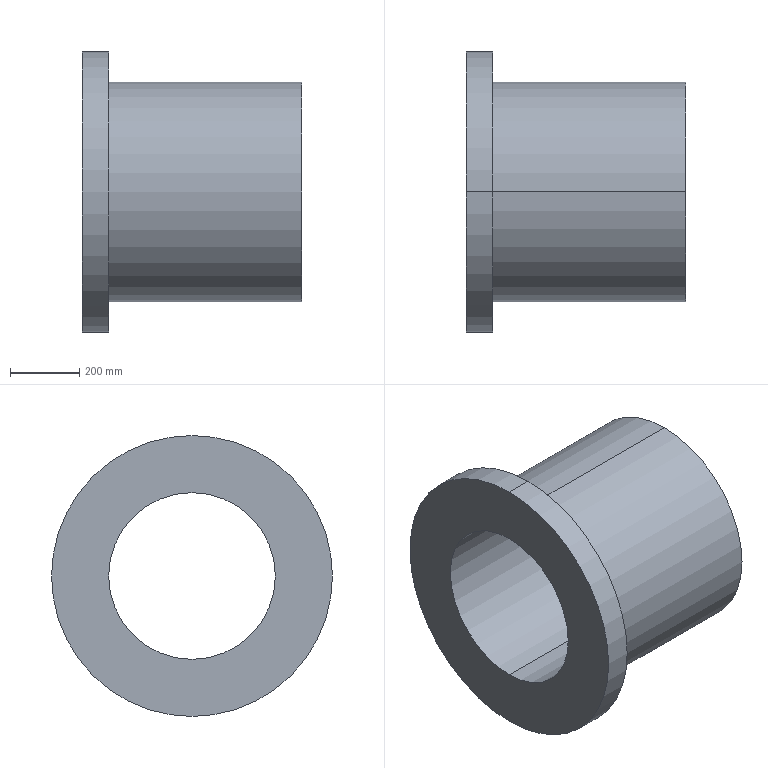Part | SolidWorks | features Revolution 1 | 1 solid | 9 faces | box 635 x 812.8 x 812.8 mm | volume 100350275 mm3 | cylinder 6 | plane 3 | commonest cylinder face diameters 482.6 x2 635 x2 812.8 x2
STEP:
#1=CARTESIAN_POINT('',(3.,0.,16.));
#2=VERTEX_POINT('',#1);
#3=CARTESIAN_POINT('',(3.,0.,-16.));
#4=VERTEX_POINT('',#3);
#5=CARTESIAN_POINT('',(3.,0.,0.));
#6=DIRECTION('',(-1.,0.,0.));
#7=DIRECTION('',(0.,0.,1.));
#8=AXIS2_PLACEMENT_3D('',#5,#6,#7);
#9=CIRCLE('',#8,16.);
#10=EDGE_CURVE('',#2,#4,#9,.T.);
#11=ORIENTED_EDGE('',*,*,#10,.T.);
#12=CARTESIAN_POINT('',(0.,0.,-16.));
#13=VERTEX_POINT('',#12);
#14=CARTESIAN_POINT('',(0.,0.,-16.));
#15=DIRECTION('',(-1.,0.,0.));
#16=VECTOR('',#15,39.37);
#17=LINE('',#14,#16);
#18=EDGE_CURVE('',#4,#13,#17,.T.);
#19=ORIENTED_EDGE('',*,*,#18,.T.);
#20=CARTESIAN_POINT('',(0.,0.,16.));
#21=VERTEX_POINT('',#20);
#22=CARTESIAN_POINT('',(0.,0.,0.));
#23=DIRECTION('',(-1.,0.,0.));
#24=DIRECTION('',(0.,0.,1.));
#25=AXIS2_PLACEMENT_3D('',#22,#23,#24);
#26=CIRCLE('',#25,16.);
#27=EDGE_CURVE('',#21,#13,#26,.T.);
#28=ORIENTED_EDGE('',*,*,#27,.F.);
#29=CARTESIAN_POINT('',(0.,0.,16.));
#30=DIRECTION('',(-1.,0.,0.));
#31=VECTOR('',#30,39.37);
#32=LINE('',#29,#31);
#33=EDGE_CURVE('',#2,#21,#32,.T.);
#34=ORIENTED_EDGE('',*,*,#33,.F.);
#35=EDGE_LOOP('',(#11,#19,#28,#34));
#36=FACE_OUTER_BOUND('',#35,.T.);
#37=CARTESIAN_POINT('',(0.,0.,0.));
#38=DIRECTION('',(-1.,0.,0.));
#39=DIRECTION('',(0.,0.,1.));
#40=AXIS2_PLACEMENT_3D('',#37,#38,#39);
#41=CYLINDRICAL_SURFACE('',#40,16.);
#42=ADVANCED_FACE('',(#36),#41,.T.);
#43=CARTESIAN_POINT('',(25.,0.,12.5));
#44=VERTEX_POINT('',#43);
#45=CARTESIAN_POINT('',(25.,0.,-12.5));
#46=VERTEX_POINT('',#45);
#47=CARTESIAN_POINT('',(25.,0.,0.));
#48=DIRECTION('',(-1.,0.,0.));
#49=DIRECTION('',(0.,0.,1.));
#50=AXIS2_PLACEMENT_3D('',#47,#48,#49);
#51=CIRCLE('',#50,12.5);
#52=EDGE_CURVE('',#44,#46,#51,.T.);
#53=ORIENTED_EDGE('',*,*,#52,.T.);
#54=CARTESIAN_POINT('',(3.,0.,-12.5));
#55=VERTEX_POINT('',#54);
#56=CARTESIAN_POINT('',(0.,0.,-12.5));
#57=DIRECTION('',(-1.,0.,0.));
#58=VECTOR('',#57,39.37);
#59=LINE('',#56,#58);
#60=EDGE_CURVE('',#46,#55,#59,.T.);
#61=ORIENTED_EDGE('',*,*,#60,.T.);
#62=CARTESIAN_POINT('',(3.,0.,12.5));
#63=VERTEX_POINT('',#62);
#64=CARTESIAN_POINT('',(3.,0.,0.));
#65=DIRECTION('',(-1.,0.,0.));
#66=DIRECTION('',(0.,0.,1.));
#67=AXIS2_PLACEMENT_3D('',#64,#65,#66);
#68=CIRCLE('',#67,12.5);
#69=EDGE_CURVE('',#63,#55,#68,.T.);
#70=ORIENTED_EDGE('',*,*,#69,.F.);
#71=CARTESIAN_POINT('',(0.,0.,12.5));
#72=DIRECTION('',(-1.,0.,0.));
#73=VECTOR('',#72,39.37);
#74=LINE('',#71,#73);
#75=EDGE_CURVE('',#44,#63,#74,.T.);
#76=ORIENTED_EDGE('',*,*,#75,.F.);
#77=EDGE_LOOP('',(#53,#61,#70,#76));
#78=FACE_OUTER_BOUND('',#77,.T.);
#79=CARTESIAN_POINT('',(0.,0.,0.));
#80=DIRECTION('',(-1.,0.,0.));
#81=DIRECTION('',(0.,0.,1.));
#82=AXIS2_PLACEMENT_3D('',#79,#80,#81);
#83=CYLINDRICAL_SURFACE('',#82,12.5);
#84=ADVANCED_FACE('',(#78),#83,.T.);
#85=CARTESIAN_POINT('',(25.,0.,-9.5));
#86=VERTEX_POINT('',#85);
#87=CARTESIAN_POINT('',(25.,0.,9.5));
#88=VERTEX_POINT('',#87);
#89=CARTESIAN_POINT('',(25.,0.,0.));
#90=DIRECTION('',(-1.,0.,0.));
#91=DIRECTION('',(0.,0.,1.));
#92=AXIS2_PLACEMENT_3D('',#89,#90,#91);
#93=CIRCLE('',#92,9.5);
#94=EDGE_CURVE('',#86,#88,#93,.T.);
#95=ORIENTED_EDGE('',*,*,#94,.F.);
#96=CARTESIAN_POINT('',(0.,0.,-9.5));
#97=VERTEX_POINT('',#96);
#98=CARTESIAN_POINT('',(0.,0.,-9.5));
#99=DIRECTION('',(-1.,0.,0.));
#100=VECTOR('',#99,39.37);
#101=LINE('',#98,#100);
#102=EDGE_CURVE('',#86,#97,#101,.T.);
#103=ORIENTED_EDGE('',*,*,#102,.T.);
#104=CARTESIAN_POINT('',(0.,0.,9.5));
#105=VERTEX_POINT('',#104);
#106=CARTESIAN_POINT('',(0.,0.,0.));
#107=DIRECTION('',(-1.,0.,0.));
#108=DIRECTION('',(0.,0.,1.));
#109=AXIS2_PLACEMENT_3D('',#106,#107,#108);
#110=CIRCLE('',#109,9.5);
#111=EDGE_CURVE('',#97,#105,#110,.T.);
#112=ORIENTED_EDGE('',*,*,#111,.T.);
#113=CARTESIAN_POINT('',(0.,0.,9.5));
#114=DIRECTION('',(-1.,0.,0.));
#115=VECTOR('',#114,39.37);
#116=LINE('',#113,#115);
#117=EDGE_CURVE('',#88,#105,#116,.T.);
#118=ORIENTED_EDGE('',*,*,#117,.F.);
#119=EDGE_LOOP('',(#95,#103,#112,#118));
#120=FACE_OUTER_BOUND('',#119,.T.);
#121=CARTESIAN_POINT('',(0.,0.,0.));
#122=DIRECTION('',(-1.,0.,0.));
#123=DIRECTION('',(0.,0.,1.));
#124=AXIS2_PLACEMENT_3D('',#121,#122,#123);
#125=CYLINDRICAL_SURFACE('',#124,9.5);
#126=ADVANCED_FACE('',(#120),#125,.F.);
#127=ORIENTED_EDGE('',*,*,#102,.F.);
#128=CARTESIAN_POINT('',(25.,0.,0.));
#129=DIRECTION('',(-1.,0.,0.));
#130=DIRECTION('',(0.,0.,1.));
#131=AXIS2_PLACEMENT_3D('',#128,#129,#130);
#132=CIRCLE('',#131,9.5);
#133=EDGE_CURVE('',#88,#86,#132,.T.);
#134=ORIENTED_EDGE('',*,*,#133,.F.);
#135=ORIENTED_EDGE('',*,*,#117,.T.);
#136=CARTESIAN_POINT('',(0.,0.,0.));
#137=DIRECTION('',(-1.,0.,0.));
#138=DIRECTION('',(0.,0.,1.));
#139=AXIS2_PLACEMENT_3D('',#136,#137,#138);
#140=CIRCLE('',#139,9.5);
#141=EDGE_CURVE('',#105,#97,#140,.T.);
#142=ORIENTED_EDGE('',*,*,#141,.T.);
#143=EDGE_LOOP('',(#127,#134,#135,#142));
#144=FACE_OUTER_BOUND('',#143,.T.);
#145=CARTESIAN_POINT('',(0.,0.,0.));
#146=DIRECTION('',(-1.,0.,0.));
#147=DIRECTION('',(0.,0.,1.));
#148=AXIS2_PLACEMENT_3D('',#145,#146,#147);
#149=CYLINDRICAL_SURFACE('',#148,9.5);
#150=ADVANCED_FACE('',(#144),#149,.F.);
#151=ORIENTED_EDGE('',*,*,#52,.F.);
#152=CARTESIAN_POINT('',(25.,0.,0.));
#153=DIRECTION('',(-1.,0.,0.));
#154=DIRECTION('',(0.,0.,1.));
#155=AXIS2_PLACEMENT_3D('',#152,#153,#154);
#156=CIRCLE('',#155,12.5);
#157=EDGE_CURVE('',#46,#44,#156,.T.);
#158=ORIENTED_EDGE('',*,*,#157,.F.);
#159=EDGE_LOOP('',(#151,#158));
#160=FACE_OUTER_BOUND('',#159,.T.);
#161=ORIENTED_EDGE('',*,*,#133,.T.);
#162=ORIENTED_EDGE('',*,*,#94,.T.);
#163=EDGE_LOOP('',(#161,#162));
#164=FACE_BOUND('',#163,.T.);
#165=CARTESIAN_POINT('',(25.,9.5,0.));
#166=DIRECTION('',(-1.,0.,0.));
#167=DIRECTION('',(0.,0.,1.));
#168=AXIS2_PLACEMENT_3D('',#165,#166,#167);
#169=PLANE('',#168);
#170=ADVANCED_FACE('',(#160,#164),#169,.F.);
#171=ORIENTED_EDGE('',*,*,#60,.F.);
#172=ORIENTED_EDGE('',*,*,#157,.T.);
#173=ORIENTED_EDGE('',*,*,#75,.T.);
#174=CARTESIAN_POINT('',(3.,0.,0.));
#175=DIRECTION('',(-1.,0.,0.));
#176=DIRECTION('',(0.,0.,1.));
#177=AXIS2_PLACEMENT_3D('',#174,#175,#176);
#178=CIRCLE('',#177,12.5);
#179=EDGE_CURVE('',#55,#63,#178,.T.);
#180=ORIENTED_EDGE('',*,*,#179,.F.);
#181=EDGE_LOOP('',(#171,#172,#173,#180));
#182=FACE_OUTER_BOUND('',#181,.T.);
#183=CARTESIAN_POINT('',(0.,0.,0.));
#184=DIRECTION('',(-1.,0.,0.));
#185=DIRECTION('',(0.,0.,1.));
#186=AXIS2_PLACEMENT_3D('',#183,#184,#185);
#187=CYLINDRICAL_SURFACE('',#186,12.5);
#188=ADVANCED_FACE('',(#182),#187,.T.);
#189=ORIENTED_EDGE('',*,*,#10,.F.);
#190=CARTESIAN_POINT('',(3.,0.,0.));
#191=DIRECTION('',(-1.,0.,0.));
#192=DIRECTION('',(0.,0.,1.));
#193=AXIS2_PLACEMENT_3D('',#190,#191,#192);
#194=CIRCLE('',#193,16.);
#195=EDGE_CURVE('',#4,#2,#194,.T.);
#196=ORIENTED_EDGE('',*,*,#195,.F.);
#197=EDGE_LOOP('',(#189,#196));
#198=FACE_OUTER_BOUND('',#197,.T.);
#199=ORIENTED_EDGE('',*,*,#69,.T.);
#200=ORIENTED_EDGE('',*,*,#179,.T.);
#201=EDGE_LOOP('',(#199,#200));
#202=FACE_BOUND('',#201,.T.);
#203=CARTESIAN_POINT('',(3.,12.5,0.));
#204=DIRECTION('',(-1.,0.,0.));
#205=DIRECTION('',(0.,0.,1.));
#206=AXIS2_PLACEMENT_3D('',#203,#204,#205);
#207=PLANE('',#206);
#208=ADVANCED_FACE('',(#198,#202),#207,.F.);
#209=ORIENTED_EDGE('',*,*,#18,.F.);
#210=ORIENTED_EDGE('',*,*,#195,.T.);
#211=ORIENTED_EDGE('',*,*,#33,.T.);
#212=CARTESIAN_POINT('',(0.,0.,0.));
#213=DIRECTION('',(-1.,0.,0.));
#214=DIRECTION('',(0.,0.,1.));
#215=AXIS2_PLACEMENT_3D('',#212,#213,#214);
#216=CIRCLE('',#215,16.);
#217=EDGE_CURVE('',#13,#21,#216,.T.);
#218=ORIENTED_EDGE('',*,*,#217,.F.);
#219=EDGE_LOOP('',(#209,#210,#211,#218));
#220=FACE_OUTER_BOUND('',#219,.T.);
#221=CARTESIAN_POINT('',(0.,0.,0.));
#222=DIRECTION('',(-1.,0.,0.));
#223=DIRECTION('',(0.,0.,1.));
#224=AXIS2_PLACEMENT_3D('',#221,#222,#223);
#225=CYLINDRICAL_SURFACE('',#224,16.);
#226=ADVANCED_FACE('',(#220),#225,.T.);
#227=ORIENTED_EDGE('',*,*,#141,.F.);
#228=ORIENTED_EDGE('',*,*,#111,.F.);
#229=EDGE_LOOP('',(#227,#228));
#230=FACE_BOUND('',#229,.T.);
#231=ORIENTED_EDGE('',*,*,#27,.T.);
#232=ORIENTED_EDGE('',*,*,#217,.T.);
#233=EDGE_LOOP('',(#231,#232));
#234=FACE_OUTER_BOUND('',#233,.T.);
#235=CARTESIAN_POINT('',(0.,9.5,0.));
#236=DIRECTION('',(1.,0.,0.));
#237=DIRECTION('',(0.,0.,-1.));
#238=AXIS2_PLACEMENT_3D('',#235,#236,#237);
#239=PLANE('',#238);
#240=ADVANCED_FACE('',(#230,#234),#239,.F.);
#241=CLOSED_SHELL('',(#42,#84,#126,#150,#170,#188,#208,#226,#240));
#242=MANIFOLD_SOLID_BREP('',#241);
#243=CARTESIAN_POINT('',(0.,0.,0.));
#244=DIRECTION('',(0.,0.,1.));
#245=DIRECTION('',(1.,0.,0.));
#246=AXIS2_PLACEMENT_3D('',#243,#244,#245);
#247=(LENGTH_UNIT()NAMED_UNIT(*)SI_UNIT($,.METRE.));
#248=LENGTH_MEASURE_WITH_UNIT(LENGTH_MEASURE(0.0254),#247);
#249=DIMENSIONAL_EXPONENTS(1.,0.,0.,0.,0.,0.,0.);
#250=(CONVERSION_BASED_UNIT('INCH',#248)LENGTH_UNIT()NAMED_UNIT(#249));
#251=UNCERTAINTY_MEASURE_WITH_UNIT(LENGTH_MEASURE(0.00001),#250,'','');
#252=(NAMED_UNIT(*)PLANE_ANGLE_UNIT()SI_UNIT($,.RADIAN.));
#253=(NAMED_UNIT(*)SI_UNIT($,.STERADIAN.)SOLID_ANGLE_UNIT());
#254=(GEOMETRIC_REPRESENTATION_CONTEXT(3)GLOBAL_UNCERTAINTY_ASSIGNED_CONTEXT((#251))GLOBAL_UNIT_ASSIGNED_CONTEXT((#250,#252,#253))REPRESENTATION_CONTEXT('',''));
#255=ADVANCED_BREP_SHAPE_REPRESENTATION('',(#242,#246),#254);